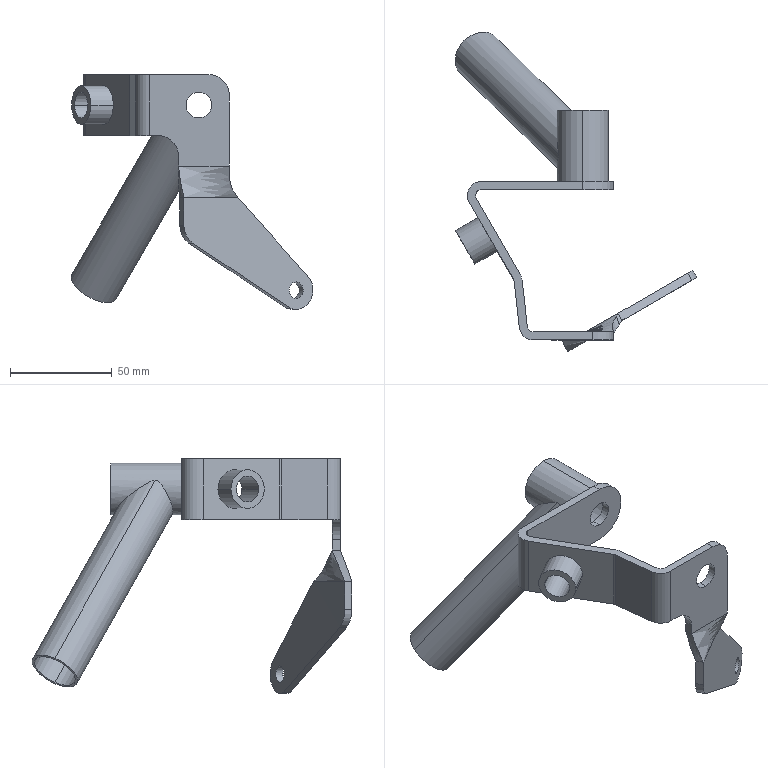Part | STEP file | KMX Cobra Front Pivot RHS | 1 solid | 60 faces | box 119.015 x 157.368 x 115.563 mm | volume 46907 mm3 | cylinder 33 | plane 21 | spline 6 | commonest cylinder face diameters 12.7 x6 19 x4 25.4 x4 6 x3 14 x3 8 x2